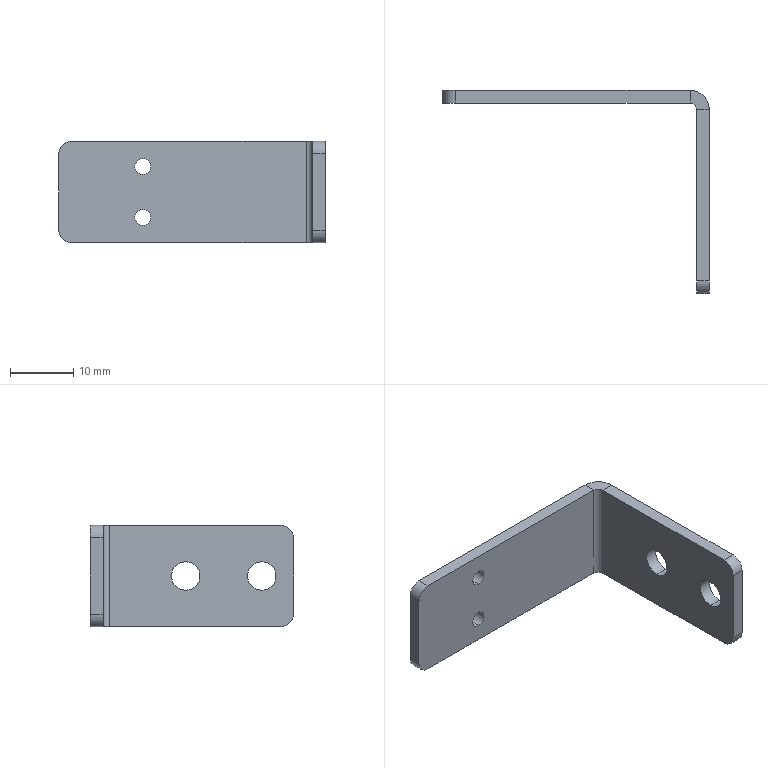Part | NX | features BREP 1 | 1 solid | 26 faces | box 42 x 32 x 16 mm | volume 2186 mm3 | cylinder 14 | plane 12 | commonest cylinder face diameters 2.5 x4 4 x4 4.5 x4 2 x1 6 x1
STEP:
#1=CARTESIAN_POINT('',(-38.,0.,8.));
#2=VERTEX_POINT('',#1);
#3=CARTESIAN_POINT('',(-40.,0.,6.));
#4=VERTEX_POINT('',#3);
#5=CARTESIAN_POINT('',(-38.,0.,6.));
#6=DIRECTION('',(0.,-1.,0.));
#7=DIRECTION('',(1.,0.,0.));
#8=AXIS2_PLACEMENT_3D('',#5,#6,#7);
#9=CIRCLE('',#8,2.);
#10=EDGE_CURVE('',#2,#4,#9,.T.);
#11=ORIENTED_EDGE('',*,*,#10,.F.);
#12=CARTESIAN_POINT('',(-38.,2.,8.));
#13=VERTEX_POINT('',#12);
#14=CARTESIAN_POINT('',(-38.,-1.,8.));
#15=DIRECTION('',(0.,-1.,0.));
#16=VECTOR('',#15,1000.);
#17=LINE('',#14,#16);
#18=EDGE_CURVE('',#13,#2,#17,.T.);
#19=ORIENTED_EDGE('',*,*,#18,.F.);
#20=CARTESIAN_POINT('',(-40.,2.,6.));
#21=VERTEX_POINT('',#20);
#22=CARTESIAN_POINT('',(-38.,2.,6.));
#23=DIRECTION('',(0.,1.,0.));
#24=DIRECTION('',(1.,0.,0.));
#25=AXIS2_PLACEMENT_3D('',#22,#23,#24);
#26=CIRCLE('',#25,2.);
#27=EDGE_CURVE('',#21,#13,#26,.T.);
#28=ORIENTED_EDGE('',*,*,#27,.F.);
#29=CARTESIAN_POINT('',(-40.,0.,6.));
#30=DIRECTION('',(0.,1.,0.));
#31=VECTOR('',#30,1000.);
#32=LINE('',#29,#31);
#33=EDGE_CURVE('',#4,#21,#32,.T.);
#34=ORIENTED_EDGE('',*,*,#33,.F.);
#35=EDGE_LOOP('',(#11,#19,#28,#34));
#36=FACE_BOUND('',#35,.T.);
#37=CARTESIAN_POINT('',(-38.,0.,6.));
#38=DIRECTION('',(0.,1.,0.));
#39=DIRECTION('',(0.,0.,1.));
#40=AXIS2_PLACEMENT_3D('',#37,#38,#39);
#41=CYLINDRICAL_SURFACE('',#40,2.);
#42=ADVANCED_FACE('',(#36),#41,.T.);
#43=CARTESIAN_POINT('',(-40.,0.,-6.));
#44=VERTEX_POINT('',#43);
#45=CARTESIAN_POINT('',(-38.,0.,-8.));
#46=VERTEX_POINT('',#45);
#47=CARTESIAN_POINT('',(-38.,0.,-6.));
#48=DIRECTION('',(0.,-1.,0.));
#49=DIRECTION('',(1.,0.,0.));
#50=AXIS2_PLACEMENT_3D('',#47,#48,#49);
#51=CIRCLE('',#50,2.);
#52=EDGE_CURVE('',#44,#46,#51,.T.);
#53=ORIENTED_EDGE('',*,*,#52,.F.);
#54=CARTESIAN_POINT('',(-40.,2.,-6.));
#55=VERTEX_POINT('',#54);
#56=CARTESIAN_POINT('',(-40.,0.,-6.));
#57=DIRECTION('',(0.,-1.,0.));
#58=VECTOR('',#57,1000.);
#59=LINE('',#56,#58);
#60=EDGE_CURVE('',#55,#44,#59,.T.);
#61=ORIENTED_EDGE('',*,*,#60,.F.);
#62=CARTESIAN_POINT('',(-38.,2.,-8.));
#63=VERTEX_POINT('',#62);
#64=CARTESIAN_POINT('',(-38.,2.,-6.));
#65=DIRECTION('',(0.,1.,0.));
#66=DIRECTION('',(1.,0.,0.));
#67=AXIS2_PLACEMENT_3D('',#64,#65,#66);
#68=CIRCLE('',#67,2.);
#69=EDGE_CURVE('',#63,#55,#68,.T.);
#70=ORIENTED_EDGE('',*,*,#69,.F.);
#71=CARTESIAN_POINT('',(-38.,-1.,-8.));
#72=DIRECTION('',(0.,1.,0.));
#73=VECTOR('',#72,1000.);
#74=LINE('',#71,#73);
#75=EDGE_CURVE('',#46,#63,#74,.T.);
#76=ORIENTED_EDGE('',*,*,#75,.F.);
#77=EDGE_LOOP('',(#53,#61,#70,#76));
#78=FACE_BOUND('',#77,.T.);
#79=CARTESIAN_POINT('',(-38.,-1.,-6.));
#80=DIRECTION('',(0.,1.,0.));
#81=DIRECTION('',(0.,0.,1.));
#82=AXIS2_PLACEMENT_3D('',#79,#80,#81);
#83=CYLINDRICAL_SURFACE('',#82,2.);
#84=ADVANCED_FACE('',(#78),#83,.T.);
#85=CARTESIAN_POINT('',(2.,-28.,8.));
#86=VERTEX_POINT('',#85);
#87=CARTESIAN_POINT('',(2.,-30.,6.));
#88=VERTEX_POINT('',#87);
#89=CARTESIAN_POINT('',(2.,-28.,6.));
#90=DIRECTION('',(1.,0.,0.));
#91=DIRECTION('',(0.,0.,1.));
#92=AXIS2_PLACEMENT_3D('',#89,#90,#91);
#93=CIRCLE('',#92,2.);
#94=EDGE_CURVE('',#86,#88,#93,.T.);
#95=ORIENTED_EDGE('',*,*,#94,.F.);
#96=CARTESIAN_POINT('',(0.,-28.,8.));
#97=VERTEX_POINT('',#96);
#98=CARTESIAN_POINT('',(2.,-28.,8.));
#99=DIRECTION('',(1.,0.,0.));
#100=VECTOR('',#99,1000.);
#101=LINE('',#98,#100);
#102=EDGE_CURVE('',#97,#86,#101,.T.);
#103=ORIENTED_EDGE('',*,*,#102,.F.);
#104=CARTESIAN_POINT('',(0.,-30.,6.));
#105=VERTEX_POINT('',#104);
#106=CARTESIAN_POINT('',(0.,-28.,6.));
#107=DIRECTION('',(-1.,0.,0.));
#108=DIRECTION('',(0.,0.,1.));
#109=AXIS2_PLACEMENT_3D('',#106,#107,#108);
#110=CIRCLE('',#109,2.);
#111=EDGE_CURVE('',#105,#97,#110,.T.);
#112=ORIENTED_EDGE('',*,*,#111,.F.);
#113=CARTESIAN_POINT('',(0.,-30.,6.));
#114=DIRECTION('',(-1.,0.,0.));
#115=VECTOR('',#114,1000.);
#116=LINE('',#113,#115);
#117=EDGE_CURVE('',#88,#105,#116,.T.);
#118=ORIENTED_EDGE('',*,*,#117,.F.);
#119=EDGE_LOOP('',(#95,#103,#112,#118));
#120=FACE_BOUND('',#119,.T.);
#121=CARTESIAN_POINT('',(2.,-28.,6.));
#122=DIRECTION('',(1.,0.,0.));
#123=DIRECTION('',(0.,0.,-1.));
#124=AXIS2_PLACEMENT_3D('',#121,#122,#123);
#125=CYLINDRICAL_SURFACE('',#124,2.);
#126=ADVANCED_FACE('',(#120),#125,.T.);
#127=CARTESIAN_POINT('',(2.,-30.,-6.));
#128=VERTEX_POINT('',#127);
#129=CARTESIAN_POINT('',(2.,-28.,-8.));
#130=VERTEX_POINT('',#129);
#131=CARTESIAN_POINT('',(2.,-28.,-6.));
#132=DIRECTION('',(1.,0.,0.));
#133=DIRECTION('',(0.,0.,1.));
#134=AXIS2_PLACEMENT_3D('',#131,#132,#133);
#135=CIRCLE('',#134,2.);
#136=EDGE_CURVE('',#128,#130,#135,.T.);
#137=ORIENTED_EDGE('',*,*,#136,.F.);
#138=CARTESIAN_POINT('',(0.,-30.,-6.));
#139=VERTEX_POINT('',#138);
#140=CARTESIAN_POINT('',(2.,-30.,-6.));
#141=DIRECTION('',(1.,0.,0.));
#142=VECTOR('',#141,1000.);
#143=LINE('',#140,#142);
#144=EDGE_CURVE('',#139,#128,#143,.T.);
#145=ORIENTED_EDGE('',*,*,#144,.F.);
#146=CARTESIAN_POINT('',(0.,-28.,-8.));
#147=VERTEX_POINT('',#146);
#148=CARTESIAN_POINT('',(0.,-28.,-6.));
#149=DIRECTION('',(-1.,0.,0.));
#150=DIRECTION('',(0.,0.,1.));
#151=AXIS2_PLACEMENT_3D('',#148,#149,#150);
#152=CIRCLE('',#151,2.);
#153=EDGE_CURVE('',#147,#139,#152,.T.);
#154=ORIENTED_EDGE('',*,*,#153,.F.);
#155=CARTESIAN_POINT('',(-1.,-28.,-8.));
#156=DIRECTION('',(-1.,0.,0.));
#157=VECTOR('',#156,1000.);
#158=LINE('',#155,#157);
#159=EDGE_CURVE('',#130,#147,#158,.T.);
#160=ORIENTED_EDGE('',*,*,#159,.F.);
#161=EDGE_LOOP('',(#137,#145,#154,#160));
#162=FACE_BOUND('',#161,.T.);
#163=CARTESIAN_POINT('',(-1.,-28.,-6.));
#164=DIRECTION('',(-1.,0.,0.));
#165=DIRECTION('',(0.,0.,1.));
#166=AXIS2_PLACEMENT_3D('',#163,#164,#165);
#167=CYLINDRICAL_SURFACE('',#166,2.);
#168=ADVANCED_FACE('',(#162),#167,.T.);
#169=CARTESIAN_POINT('',(0.,-13.,-2.25));
#170=VERTEX_POINT('',#169);
#171=CARTESIAN_POINT('',(2.,-13.,-2.25));
#172=VERTEX_POINT('',#171);
#173=CARTESIAN_POINT('',(0.,-13.,-2.25));
#174=DIRECTION('',(-1.,0.,0.));
#175=VECTOR('',#174,1000.);
#176=LINE('',#173,#175);
#177=EDGE_CURVE('',#170,#172,#176,.F.);
#178=ORIENTED_EDGE('',*,*,#177,.T.);
#179=CARTESIAN_POINT('',(2.,-13.,2.25));
#180=VERTEX_POINT('',#179);
#181=CARTESIAN_POINT('',(2.,-13.,0.));
#182=DIRECTION('',(-1.,0.,0.));
#183=DIRECTION('',(0.,0.,1.));
#184=AXIS2_PLACEMENT_3D('',#181,#182,#183);
#185=CIRCLE('',#184,2.25);
#186=EDGE_CURVE('',#180,#172,#185,.T.);
#187=ORIENTED_EDGE('',*,*,#186,.F.);
#188=CARTESIAN_POINT('',(0.,-13.,2.25));
#189=VERTEX_POINT('',#188);
#190=CARTESIAN_POINT('',(0.,-13.,2.25));
#191=DIRECTION('',(-1.,0.,0.));
#192=VECTOR('',#191,1000.);
#193=LINE('',#190,#192);
#194=EDGE_CURVE('',#189,#180,#193,.F.);
#195=ORIENTED_EDGE('',*,*,#194,.F.);
#196=CARTESIAN_POINT('',(0.,-13.,0.));
#197=DIRECTION('',(-1.,0.,0.));
#198=DIRECTION('',(0.,0.,1.));
#199=AXIS2_PLACEMENT_3D('',#196,#197,#198);
#200=CIRCLE('',#199,2.25);
#201=EDGE_CURVE('',#189,#170,#200,.T.);
#202=ORIENTED_EDGE('',*,*,#201,.T.);
#203=EDGE_LOOP('',(#178,#187,#195,#202));
#204=FACE_BOUND('',#203,.T.);
#205=CARTESIAN_POINT('',(0.,-13.,0.));
#206=DIRECTION('',(-1.,0.,0.));
#207=DIRECTION('',(0.,0.,1.));
#208=AXIS2_PLACEMENT_3D('',#205,#206,#207);
#209=CYLINDRICAL_SURFACE('',#208,2.25);
#210=ADVANCED_FACE('',(#204),#209,.F.);
#211=CARTESIAN_POINT('',(0.,-25.,-2.25));
#212=VERTEX_POINT('',#211);
#213=CARTESIAN_POINT('',(2.,-25.,-2.25));
#214=VERTEX_POINT('',#213);
#215=CARTESIAN_POINT('',(0.,-25.,-2.25));
#216=DIRECTION('',(-1.,0.,0.));
#217=VECTOR('',#216,1000.);
#218=LINE('',#215,#217);
#219=EDGE_CURVE('',#212,#214,#218,.F.);
#220=ORIENTED_EDGE('',*,*,#219,.T.);
#221=CARTESIAN_POINT('',(2.,-25.,2.25));
#222=VERTEX_POINT('',#221);
#223=CARTESIAN_POINT('',(2.,-25.,0.));
#224=DIRECTION('',(-1.,0.,0.));
#225=DIRECTION('',(0.,0.,1.));
#226=AXIS2_PLACEMENT_3D('',#223,#224,#225);
#227=CIRCLE('',#226,2.25);
#228=EDGE_CURVE('',#222,#214,#227,.T.);
#229=ORIENTED_EDGE('',*,*,#228,.F.);
#230=CARTESIAN_POINT('',(0.,-25.,2.25));
#231=VERTEX_POINT('',#230);
#232=CARTESIAN_POINT('',(0.,-25.,2.25));
#233=DIRECTION('',(-1.,0.,0.));
#234=VECTOR('',#233,1000.);
#235=LINE('',#232,#234);
#236=EDGE_CURVE('',#231,#222,#235,.F.);
#237=ORIENTED_EDGE('',*,*,#236,.F.);
#238=CARTESIAN_POINT('',(0.,-25.,0.));
#239=DIRECTION('',(-1.,0.,0.));
#240=DIRECTION('',(0.,0.,1.));
#241=AXIS2_PLACEMENT_3D('',#238,#239,#240);
#242=CIRCLE('',#241,2.25);
#243=EDGE_CURVE('',#231,#212,#242,.T.);
#244=ORIENTED_EDGE('',*,*,#243,.T.);
#245=EDGE_LOOP('',(#220,#229,#237,#244));
#246=FACE_BOUND('',#245,.T.);
#247=CARTESIAN_POINT('',(0.,-25.,0.));
#248=DIRECTION('',(-1.,0.,0.));
#249=DIRECTION('',(0.,0.,1.));
#250=AXIS2_PLACEMENT_3D('',#247,#248,#249);
#251=CYLINDRICAL_SURFACE('',#250,2.25);
#252=ADVANCED_FACE('',(#246),#251,.F.);
#253=CARTESIAN_POINT('',(-26.75,2.,2.75));
#254=VERTEX_POINT('',#253);
#255=CARTESIAN_POINT('',(-26.75,0.,2.75));
#256=VERTEX_POINT('',#255);
#257=CARTESIAN_POINT('',(-26.75,2.,2.75));
#258=DIRECTION('',(0.,1.,0.));
#259=VECTOR('',#258,1000.);
#260=LINE('',#257,#259);
#261=EDGE_CURVE('',#254,#256,#260,.F.);
#262=ORIENTED_EDGE('',*,*,#261,.T.);
#263=CARTESIAN_POINT('',(-26.75,0.,5.25));
#264=VERTEX_POINT('',#263);
#265=CARTESIAN_POINT('',(-26.75,0.,4.));
#266=DIRECTION('',(0.,-1.,0.));
#267=DIRECTION('',(1.,0.,0.));
#268=AXIS2_PLACEMENT_3D('',#265,#266,#267);
#269=CIRCLE('',#268,1.25);
#270=EDGE_CURVE('',#256,#264,#269,.T.);
#271=ORIENTED_EDGE('',*,*,#270,.T.);
#272=CARTESIAN_POINT('',(-26.75,2.,5.25));
#273=VERTEX_POINT('',#272);
#274=CARTESIAN_POINT('',(-26.75,2.,5.25));
#275=DIRECTION('',(0.,1.,0.));
#276=VECTOR('',#275,1000.);
#277=LINE('',#274,#276);
#278=EDGE_CURVE('',#273,#264,#277,.F.);
#279=ORIENTED_EDGE('',*,*,#278,.F.);
#280=CARTESIAN_POINT('',(-26.75,2.,4.));
#281=DIRECTION('',(0.,1.,0.));
#282=DIRECTION('',(0.,0.,1.));
#283=AXIS2_PLACEMENT_3D('',#280,#281,#282);
#284=CIRCLE('',#283,1.25);
#285=EDGE_CURVE('',#273,#254,#284,.T.);
#286=ORIENTED_EDGE('',*,*,#285,.T.);
#287=EDGE_LOOP('',(#262,#271,#279,#286));
#288=FACE_BOUND('',#287,.T.);
#289=CARTESIAN_POINT('',(-26.75,2.,4.));
#290=DIRECTION('',(0.,1.,0.));
#291=DIRECTION('',(0.,0.,1.));
#292=AXIS2_PLACEMENT_3D('',#289,#290,#291);
#293=CYLINDRICAL_SURFACE('',#292,1.25);
#294=ADVANCED_FACE('',(#288),#293,.F.);
#295=CARTESIAN_POINT('',(-26.75,2.,-5.25));
#296=VERTEX_POINT('',#295);
#297=CARTESIAN_POINT('',(-26.75,0.,-5.25));
#298=VERTEX_POINT('',#297);
#299=CARTESIAN_POINT('',(-26.75,2.,-5.25));
#300=DIRECTION('',(0.,1.,0.));
#301=VECTOR('',#300,1000.);
#302=LINE('',#299,#301);
#303=EDGE_CURVE('',#296,#298,#302,.F.);
#304=ORIENTED_EDGE('',*,*,#303,.T.);
#305=CARTESIAN_POINT('',(-26.75,0.,-2.75));
#306=VERTEX_POINT('',#305);
#307=CARTESIAN_POINT('',(-26.75,0.,-4.));
#308=DIRECTION('',(0.,-1.,0.));
#309=DIRECTION('',(1.,0.,0.));
#310=AXIS2_PLACEMENT_3D('',#307,#308,#309);
#311=CIRCLE('',#310,1.25);
#312=EDGE_CURVE('',#298,#306,#311,.T.);
#313=ORIENTED_EDGE('',*,*,#312,.T.);
#314=CARTESIAN_POINT('',(-26.75,2.,-2.75));
#315=VERTEX_POINT('',#314);
#316=CARTESIAN_POINT('',(-26.75,2.,-2.75));
#317=DIRECTION('',(0.,1.,0.));
#318=VECTOR('',#317,1000.);
#319=LINE('',#316,#318);
#320=EDGE_CURVE('',#315,#306,#319,.F.);
#321=ORIENTED_EDGE('',*,*,#320,.F.);
#322=CARTESIAN_POINT('',(-26.75,2.,-4.));
#323=DIRECTION('',(0.,1.,0.));
#324=DIRECTION('',(0.,0.,1.));
#325=AXIS2_PLACEMENT_3D('',#322,#323,#324);
#326=CIRCLE('',#325,1.25);
#327=EDGE_CURVE('',#315,#296,#326,.T.);
#328=ORIENTED_EDGE('',*,*,#327,.T.);
#329=EDGE_LOOP('',(#304,#313,#321,#328));
#330=FACE_BOUND('',#329,.T.);
#331=CARTESIAN_POINT('',(-26.75,2.,-4.));
#332=DIRECTION('',(0.,1.,0.));
#333=DIRECTION('',(0.,0.,1.));
#334=AXIS2_PLACEMENT_3D('',#331,#332,#333);
#335=CYLINDRICAL_SURFACE('',#334,1.25);
#336=ADVANCED_FACE('',(#330),#335,.F.);
#337=CARTESIAN_POINT('',(-1.,0.,-8.));
#338=VERTEX_POINT('',#337);
#339=CARTESIAN_POINT('',(0.,0.,-8.));
#340=DIRECTION('',(-1.,0.,0.));
#341=VECTOR('',#340,1000.);
#342=LINE('',#339,#341);
#343=EDGE_CURVE('',#338,#46,#342,.T.);
#344=ORIENTED_EDGE('',*,*,#343,.T.);
#345=ORIENTED_EDGE('',*,*,#75,.T.);
#346=CARTESIAN_POINT('',(-1.,2.,-8.));
#347=VERTEX_POINT('',#346);
#348=CARTESIAN_POINT('',(0.,2.,-8.));
#349=DIRECTION('',(-1.,0.,0.));
#350=VECTOR('',#349,1000.);
#351=LINE('',#348,#350);
#352=EDGE_CURVE('',#347,#63,#351,.T.);
#353=ORIENTED_EDGE('',*,*,#352,.F.);
#354=CARTESIAN_POINT('',(-1.,2.,-8.));
#355=DIRECTION('',(0.,-1.,0.));
#356=VECTOR('',#355,1000.);
#357=LINE('',#354,#356);
#358=EDGE_CURVE('',#347,#338,#357,.T.);
#359=ORIENTED_EDGE('',*,*,#358,.T.);
#360=EDGE_LOOP('',(#344,#345,#353,#359));
#361=FACE_BOUND('',#360,.T.);
#362=CARTESIAN_POINT('',(-1.,-1.,-8.));
#363=DIRECTION('',(0.,0.,-1.));
#364=DIRECTION('',(-1.,0.,0.));
#365=AXIS2_PLACEMENT_3D('',#362,#363,#364);
#366=PLANE('',#365);
#367=ADVANCED_FACE('',(#361),#366,.T.);
#368=CARTESIAN_POINT('',(0.,-1.,8.));
#369=VERTEX_POINT('',#368);
#370=CARTESIAN_POINT('',(0.,0.,8.));
#371=DIRECTION('',(0.,1.,0.));
#372=VECTOR('',#371,1000.);
#373=LINE('',#370,#372);
#374=EDGE_CURVE('',#97,#369,#373,.T.);
#375=ORIENTED_EDGE('',*,*,#374,.F.);
#376=ORIENTED_EDGE('',*,*,#102,.T.);
#377=CARTESIAN_POINT('',(2.,-1.,8.));
#378=VERTEX_POINT('',#377);
#379=CARTESIAN_POINT('',(2.,0.,8.));
#380=DIRECTION('',(0.,1.,0.));
#381=VECTOR('',#380,1000.);
#382=LINE('',#379,#381);
#383=EDGE_CURVE('',#86,#378,#382,.T.);
#384=ORIENTED_EDGE('',*,*,#383,.T.);
#385=CARTESIAN_POINT('',(2.,-1.,8.));
#386=DIRECTION('',(-1.,0.,0.));
#387=VECTOR('',#386,1000.);
#388=LINE('',#385,#387);
#389=EDGE_CURVE('',#378,#369,#388,.T.);
#390=ORIENTED_EDGE('',*,*,#389,.T.);
#391=EDGE_LOOP('',(#375,#376,#384,#390));
#392=FACE_BOUND('',#391,.T.);
#393=CARTESIAN_POINT('',(-1.,-1.,8.));
#394=DIRECTION('',(0.,0.,-1.));
#395=DIRECTION('',(-1.,0.,0.));
#396=AXIS2_PLACEMENT_3D('',#393,#394,#395);
#397=PLANE('',#396);
#398=ADVANCED_FACE('',(#392),#397,.F.);
#399=CARTESIAN_POINT('',(2.,-1.,-8.));
#400=VERTEX_POINT('',#399);
#401=CARTESIAN_POINT('',(-1.,-1.,-8.));
#402=DIRECTION('',(0.,0.,1.));
#403=DIRECTION('',(1.,0.,0.));
#404=AXIS2_PLACEMENT_3D('',#401,#402,#403);
#405=CIRCLE('',#404,3.);
#406=EDGE_CURVE('',#400,#347,#405,.T.);
#407=ORIENTED_EDGE('',*,*,#406,.T.);
#408=CARTESIAN_POINT('',(-1.,2.,8.));
#409=VERTEX_POINT('',#408);
#410=CARTESIAN_POINT('',(-1.,2.,8.));
#411=DIRECTION('',(0.,0.,-1.));
#412=VECTOR('',#411,1000.);
#413=LINE('',#410,#412);
#414=EDGE_CURVE('',#409,#347,#413,.T.);
#415=ORIENTED_EDGE('',*,*,#414,.F.);
#416=CARTESIAN_POINT('',(-1.,-1.,8.));
#417=DIRECTION('',(0.,0.,1.));
#418=DIRECTION('',(1.,0.,0.));
#419=AXIS2_PLACEMENT_3D('',#416,#417,#418);
#420=CIRCLE('',#419,3.);
#421=EDGE_CURVE('',#378,#409,#420,.T.);
#422=ORIENTED_EDGE('',*,*,#421,.F.);
#423=CARTESIAN_POINT('',(2.,-1.,8.));
#424=DIRECTION('',(0.,0.,-1.));
#425=VECTOR('',#424,1000.);
#426=LINE('',#423,#425);
#427=EDGE_CURVE('',#378,#400,#426,.T.);
#428=ORIENTED_EDGE('',*,*,#427,.T.);
#429=EDGE_LOOP('',(#407,#415,#422,#428));
#430=FACE_BOUND('',#429,.T.);
#431=CARTESIAN_POINT('',(-1.,-1.,8.));
#432=DIRECTION('',(0.,0.,-1.));
#433=DIRECTION('',(-1.,0.,0.));
#434=AXIS2_PLACEMENT_3D('',#431,#432,#433);
#435=CYLINDRICAL_SURFACE('',#434,3.);
#436=ADVANCED_FACE('',(#430),#435,.T.);
#437=CARTESIAN_POINT('',(2.,-30.,8.));
#438=DIRECTION('',(0.,0.,-1.));
#439=VECTOR('',#438,1000.);
#440=LINE('',#437,#439);
#441=EDGE_CURVE('',#88,#128,#440,.T.);
#442=ORIENTED_EDGE('',*,*,#441,.T.);
#443=ORIENTED_EDGE('',*,*,#136,.T.);
#444=CARTESIAN_POINT('',(2.,0.,-8.));
#445=DIRECTION('',(0.,1.,0.));
#446=VECTOR('',#445,1000.);
#447=LINE('',#444,#446);
#448=EDGE_CURVE('',#130,#400,#447,.T.);
#449=ORIENTED_EDGE('',*,*,#448,.T.);
#450=ORIENTED_EDGE('',*,*,#427,.F.);
#451=ORIENTED_EDGE('',*,*,#383,.F.);
#452=ORIENTED_EDGE('',*,*,#94,.T.);
#453=EDGE_LOOP('',(#442,#443,#449,#450,#451,#452));
#454=FACE_BOUND('',#453,.T.);
#455=ORIENTED_EDGE('',*,*,#228,.T.);
#456=CARTESIAN_POINT('',(2.,-25.,0.));
#457=DIRECTION('',(-1.,0.,0.));
#458=DIRECTION('',(0.,0.,1.));
#459=AXIS2_PLACEMENT_3D('',#456,#457,#458);
#460=CIRCLE('',#459,2.25);
#461=EDGE_CURVE('',#214,#222,#460,.T.);
#462=ORIENTED_EDGE('',*,*,#461,.T.);
#463=EDGE_LOOP('',(#455,#462));
#464=FACE_BOUND('',#463,.T.);
#465=ORIENTED_EDGE('',*,*,#186,.T.);
#466=CARTESIAN_POINT('',(2.,-13.,0.));
#467=DIRECTION('',(-1.,0.,0.));
#468=DIRECTION('',(0.,0.,1.));
#469=AXIS2_PLACEMENT_3D('',#466,#467,#468);
#470=CIRCLE('',#469,2.25);
#471=EDGE_CURVE('',#172,#180,#470,.T.);
#472=ORIENTED_EDGE('',*,*,#471,.T.);
#473=EDGE_LOOP('',(#465,#472));
#474=FACE_BOUND('',#473,.T.);
#475=CARTESIAN_POINT('',(2.,0.,8.));
#476=DIRECTION('',(-1.,0.,0.));
#477=DIRECTION('',(0.,0.,1.));
#478=AXIS2_PLACEMENT_3D('',#475,#476,#477);
#479=PLANE('',#478);
#480=ADVANCED_FACE('',(#454,#464,#474),#479,.F.);
#481=CARTESIAN_POINT('',(0.,-30.,8.));
#482=DIRECTION('',(0.,0.,-1.));
#483=VECTOR('',#482,1000.);
#484=LINE('',#481,#483);
#485=EDGE_CURVE('',#105,#139,#484,.T.);
#486=ORIENTED_EDGE('',*,*,#485,.T.);
#487=ORIENTED_EDGE('',*,*,#144,.T.);
#488=ORIENTED_EDGE('',*,*,#441,.F.);
#489=ORIENTED_EDGE('',*,*,#117,.T.);
#490=EDGE_LOOP('',(#486,#487,#488,#489));
#491=FACE_BOUND('',#490,.T.);
#492=CARTESIAN_POINT('',(2.,-30.,8.));
#493=DIRECTION('',(0.,-1.,0.));
#494=DIRECTION('',(0.,0.,-1.));
#495=AXIS2_PLACEMENT_3D('',#492,#493,#494);
#496=PLANE('',#495);
#497=ADVANCED_FACE('',(#491),#496,.T.);
#498=CARTESIAN_POINT('',(0.,-1.,-8.));
#499=VERTEX_POINT('',#498);
#500=CARTESIAN_POINT('',(0.,0.,-8.));
#501=DIRECTION('',(0.,1.,0.));
#502=VECTOR('',#501,1000.);
#503=LINE('',#500,#502);
#504=EDGE_CURVE('',#147,#499,#503,.T.);
#505=ORIENTED_EDGE('',*,*,#504,.F.);
#506=ORIENTED_EDGE('',*,*,#153,.T.);
#507=ORIENTED_EDGE('',*,*,#485,.F.);
#508=ORIENTED_EDGE('',*,*,#111,.T.);
#509=ORIENTED_EDGE('',*,*,#374,.T.);
#510=CARTESIAN_POINT('',(0.,-1.,8.));
#511=DIRECTION('',(0.,0.,-1.));
#512=VECTOR('',#511,1000.);
#513=LINE('',#510,#512);
#514=EDGE_CURVE('',#369,#499,#513,.T.);
#515=ORIENTED_EDGE('',*,*,#514,.T.);
#516=EDGE_LOOP('',(#505,#506,#507,#508,#509,#515));
#517=FACE_BOUND('',#516,.T.);
#518=ORIENTED_EDGE('',*,*,#243,.F.);
#519=CARTESIAN_POINT('',(0.,-25.,0.));
#520=DIRECTION('',(-1.,0.,0.));
#521=DIRECTION('',(0.,0.,1.));
#522=AXIS2_PLACEMENT_3D('',#519,#520,#521);
#523=CIRCLE('',#522,2.25);
#524=EDGE_CURVE('',#212,#231,#523,.T.);
#525=ORIENTED_EDGE('',*,*,#524,.F.);
#526=EDGE_LOOP('',(#518,#525));
#527=FACE_BOUND('',#526,.T.);
#528=ORIENTED_EDGE('',*,*,#201,.F.);
#529=CARTESIAN_POINT('',(0.,-13.,0.));
#530=DIRECTION('',(-1.,0.,0.));
#531=DIRECTION('',(0.,0.,1.));
#532=AXIS2_PLACEMENT_3D('',#529,#530,#531);
#533=CIRCLE('',#532,2.25);
#534=EDGE_CURVE('',#170,#189,#533,.T.);
#535=ORIENTED_EDGE('',*,*,#534,.F.);
#536=EDGE_LOOP('',(#528,#535));
#537=FACE_BOUND('',#536,.T.);
#538=CARTESIAN_POINT('',(0.,0.,8.));
#539=DIRECTION('',(-1.,0.,0.));
#540=DIRECTION('',(0.,0.,1.));
#541=AXIS2_PLACEMENT_3D('',#538,#539,#540);
#542=PLANE('',#541);
#543=ADVANCED_FACE('',(#517,#527,#537),#542,.T.);
#544=CARTESIAN_POINT('',(-1.,-1.,-8.));
#545=DIRECTION('',(0.,0.,1.));
#546=DIRECTION('',(-1.,0.,0.));
#547=AXIS2_PLACEMENT_3D('',#544,#545,#546);
#548=CIRCLE('',#547,1.);
#549=EDGE_CURVE('',#499,#338,#548,.T.);
#550=ORIENTED_EDGE('',*,*,#549,.F.);
#551=ORIENTED_EDGE('',*,*,#514,.F.);
#552=CARTESIAN_POINT('',(-1.,0.,8.));
#553=VERTEX_POINT('',#552);
#554=CARTESIAN_POINT('',(-1.,-1.,8.));
#555=DIRECTION('',(0.,0.,1.));
#556=DIRECTION('',(-1.,0.,0.));
#557=AXIS2_PLACEMENT_3D('',#554,#555,#556);
#558=CIRCLE('',#557,1.);
#559=EDGE_CURVE('',#369,#553,#558,.T.);
#560=ORIENTED_EDGE('',*,*,#559,.T.);
#561=CARTESIAN_POINT('',(-1.,0.,8.));
#562=DIRECTION('',(0.,0.,-1.));
#563=VECTOR('',#562,1000.);
#564=LINE('',#561,#563);
#565=EDGE_CURVE('',#553,#338,#564,.T.);
#566=ORIENTED_EDGE('',*,*,#565,.T.);
#567=EDGE_LOOP('',(#550,#551,#560,#566));
#568=FACE_BOUND('',#567,.T.);
#569=CARTESIAN_POINT('',(-1.,-1.,8.));
#570=DIRECTION('',(0.,0.,-1.));
#571=DIRECTION('',(-1.,0.,0.));
#572=AXIS2_PLACEMENT_3D('',#569,#570,#571);
#573=CYLINDRICAL_SURFACE('',#572,1.);
#574=ADVANCED_FACE('',(#568),#573,.F.);
#575=CARTESIAN_POINT('',(-40.,0.,8.));
#576=DIRECTION('',(0.,0.,-1.));
#577=VECTOR('',#576,1000.);
#578=LINE('',#575,#577);
#579=EDGE_CURVE('',#4,#44,#578,.T.);
#580=ORIENTED_EDGE('',*,*,#579,.T.);
#581=ORIENTED_EDGE('',*,*,#52,.T.);
#582=ORIENTED_EDGE('',*,*,#343,.F.);
#583=ORIENTED_EDGE('',*,*,#565,.F.);
#584=CARTESIAN_POINT('',(0.,0.,8.));
#585=DIRECTION('',(-1.,0.,0.));
#586=VECTOR('',#585,1000.);
#587=LINE('',#584,#586);
#588=EDGE_CURVE('',#553,#2,#587,.T.);
#589=ORIENTED_EDGE('',*,*,#588,.T.);
#590=ORIENTED_EDGE('',*,*,#10,.T.);
#591=EDGE_LOOP('',(#580,#581,#582,#583,#589,#590));
#592=FACE_BOUND('',#591,.T.);
#593=CARTESIAN_POINT('',(-26.75,0.,-4.));
#594=DIRECTION('',(0.,-1.,0.));
#595=DIRECTION('',(1.,0.,0.));
#596=AXIS2_PLACEMENT_3D('',#593,#594,#595);
#597=CIRCLE('',#596,1.25);
#598=EDGE_CURVE('',#306,#298,#597,.T.);
#599=ORIENTED_EDGE('',*,*,#598,.F.);
#600=ORIENTED_EDGE('',*,*,#312,.F.);
#601=EDGE_LOOP('',(#599,#600));
#602=FACE_BOUND('',#601,.T.);
#603=CARTESIAN_POINT('',(-26.75,0.,4.));
#604=DIRECTION('',(0.,-1.,0.));
#605=DIRECTION('',(1.,0.,0.));
#606=AXIS2_PLACEMENT_3D('',#603,#604,#605);
#607=CIRCLE('',#606,1.25);
#608=EDGE_CURVE('',#264,#256,#607,.T.);
#609=ORIENTED_EDGE('',*,*,#608,.F.);
#610=ORIENTED_EDGE('',*,*,#270,.F.);
#611=EDGE_LOOP('',(#609,#610));
#612=FACE_BOUND('',#611,.T.);
#613=CARTESIAN_POINT('',(0.,0.,8.));
#614=DIRECTION('',(0.,-1.,0.));
#615=DIRECTION('',(1.,0.,0.));
#616=AXIS2_PLACEMENT_3D('',#613,#614,#615);
#617=PLANE('',#616);
#618=ADVANCED_FACE('',(#592,#602,#612),#617,.T.);
#619=CARTESIAN_POINT('',(-40.,2.,8.));
#620=DIRECTION('',(0.,0.,-1.));
#621=VECTOR('',#620,1000.);
#622=LINE('',#619,#621);
#623=EDGE_CURVE('',#21,#55,#622,.T.);
#624=ORIENTED_EDGE('',*,*,#623,.T.);
#625=ORIENTED_EDGE('',*,*,#60,.T.);
#626=ORIENTED_EDGE('',*,*,#579,.F.);
#627=ORIENTED_EDGE('',*,*,#33,.T.);
#628=EDGE_LOOP('',(#624,#625,#626,#627));
#629=FACE_BOUND('',#628,.T.);
#630=CARTESIAN_POINT('',(-40.,0.,8.));
#631=DIRECTION('',(-1.,0.,0.));
#632=DIRECTION('',(0.,0.,1.));
#633=AXIS2_PLACEMENT_3D('',#630,#631,#632);
#634=PLANE('',#633);
#635=ADVANCED_FACE('',(#629),#634,.T.);
#636=ORIENTED_EDGE('',*,*,#352,.T.);
#637=ORIENTED_EDGE('',*,*,#69,.T.);
#638=ORIENTED_EDGE('',*,*,#623,.F.);
#639=ORIENTED_EDGE('',*,*,#27,.T.);
#640=CARTESIAN_POINT('',(0.,2.,8.));
#641=DIRECTION('',(-1.,0.,0.));
#642=VECTOR('',#641,1000.);
#643=LINE('',#640,#642);
#644=EDGE_CURVE('',#409,#13,#643,.T.);
#645=ORIENTED_EDGE('',*,*,#644,.F.);
#646=ORIENTED_EDGE('',*,*,#414,.T.);
#647=EDGE_LOOP('',(#636,#637,#638,#639,#645,#646));
#648=FACE_BOUND('',#647,.T.);
#649=ORIENTED_EDGE('',*,*,#327,.F.);
#650=CARTESIAN_POINT('',(-26.75,2.,-4.));
#651=DIRECTION('',(0.,1.,0.));
#652=DIRECTION('',(0.,0.,1.));
#653=AXIS2_PLACEMENT_3D('',#650,#651,#652);
#654=CIRCLE('',#653,1.25);
#655=EDGE_CURVE('',#296,#315,#654,.T.);
#656=ORIENTED_EDGE('',*,*,#655,.F.);
#657=EDGE_LOOP('',(#649,#656));
#658=FACE_BOUND('',#657,.T.);
#659=ORIENTED_EDGE('',*,*,#285,.F.);
#660=CARTESIAN_POINT('',(-26.75,2.,4.));
#661=DIRECTION('',(0.,1.,0.));
#662=DIRECTION('',(0.,0.,1.));
#663=AXIS2_PLACEMENT_3D('',#660,#661,#662);
#664=CIRCLE('',#663,1.25);
#665=EDGE_CURVE('',#254,#273,#664,.T.);
#666=ORIENTED_EDGE('',*,*,#665,.F.);
#667=EDGE_LOOP('',(#659,#666));
#668=FACE_BOUND('',#667,.T.);
#669=CARTESIAN_POINT('',(0.,2.,8.));
#670=DIRECTION('',(0.,-1.,0.));
#671=DIRECTION('',(1.,0.,0.));
#672=AXIS2_PLACEMENT_3D('',#669,#670,#671);
#673=PLANE('',#672);
#674=ADVANCED_FACE('',(#648,#658,#668),#673,.F.);
#675=ORIENTED_EDGE('',*,*,#448,.F.);
#676=ORIENTED_EDGE('',*,*,#159,.T.);
#677=ORIENTED_EDGE('',*,*,#504,.T.);
#678=CARTESIAN_POINT('',(0.,-1.,-8.));
#679=DIRECTION('',(1.,0.,0.));
#680=VECTOR('',#679,1000.);
#681=LINE('',#678,#680);
#682=EDGE_CURVE('',#499,#400,#681,.T.);
#683=ORIENTED_EDGE('',*,*,#682,.T.);
#684=EDGE_LOOP('',(#675,#676,#677,#683));
#685=FACE_BOUND('',#684,.T.);
#686=CARTESIAN_POINT('',(-1.,2.,-8.));
#687=DIRECTION('',(0.,0.,-1.));
#688=DIRECTION('',(-1.,0.,0.));
#689=AXIS2_PLACEMENT_3D('',#686,#687,#688);
#690=PLANE('',#689);
#691=ADVANCED_FACE('',(#685),#690,.T.);
#692=ORIENTED_EDGE('',*,*,#682,.F.);
#693=ORIENTED_EDGE('',*,*,#549,.T.);
#694=ORIENTED_EDGE('',*,*,#358,.F.);
#695=ORIENTED_EDGE('',*,*,#406,.F.);
#696=EDGE_LOOP('',(#692,#693,#694,#695));
#697=FACE_BOUND('',#696,.T.);
#698=CARTESIAN_POINT('',(0.,-1.,-8.));
#699=DIRECTION('',(0.,0.,-1.));
#700=DIRECTION('',(-1.,0.,0.));
#701=AXIS2_PLACEMENT_3D('',#698,#699,#700);
#702=PLANE('',#701);
#703=ADVANCED_FACE('',(#697),#702,.T.);
#704=ORIENTED_EDGE('',*,*,#644,.T.);
#705=ORIENTED_EDGE('',*,*,#18,.T.);
#706=ORIENTED_EDGE('',*,*,#588,.F.);
#707=CARTESIAN_POINT('',(-1.,0.,8.));
#708=DIRECTION('',(0.,1.,0.));
#709=VECTOR('',#708,1000.);
#710=LINE('',#707,#709);
#711=EDGE_CURVE('',#553,#409,#710,.T.);
#712=ORIENTED_EDGE('',*,*,#711,.T.);
#713=EDGE_LOOP('',(#704,#705,#706,#712));
#714=FACE_BOUND('',#713,.T.);
#715=CARTESIAN_POINT('',(2.,-1.,8.));
#716=DIRECTION('',(0.,0.,1.));
#717=DIRECTION('',(1.,0.,0.));
#718=AXIS2_PLACEMENT_3D('',#715,#716,#717);
#719=PLANE('',#718);
#720=ADVANCED_FACE('',(#714),#719,.T.);
#721=ORIENTED_EDGE('',*,*,#711,.F.);
#722=ORIENTED_EDGE('',*,*,#559,.F.);
#723=ORIENTED_EDGE('',*,*,#389,.F.);
#724=ORIENTED_EDGE('',*,*,#421,.T.);
#725=EDGE_LOOP('',(#721,#722,#723,#724));
#726=FACE_BOUND('',#725,.T.);
#727=CARTESIAN_POINT('',(-1.,0.,8.));
#728=DIRECTION('',(0.,0.,1.));
#729=DIRECTION('',(1.,0.,0.));
#730=AXIS2_PLACEMENT_3D('',#727,#728,#729);
#731=PLANE('',#730);
#732=ADVANCED_FACE('',(#726),#731,.T.);
#733=ORIENTED_EDGE('',*,*,#598,.T.);
#734=ORIENTED_EDGE('',*,*,#303,.F.);
#735=ORIENTED_EDGE('',*,*,#655,.T.);
#736=ORIENTED_EDGE('',*,*,#320,.T.);
#737=EDGE_LOOP('',(#733,#734,#735,#736));
#738=FACE_BOUND('',#737,.T.);
#739=CARTESIAN_POINT('',(-26.75,2.,-4.));
#740=DIRECTION('',(0.,1.,0.));
#741=DIRECTION('',(0.,0.,1.));
#742=AXIS2_PLACEMENT_3D('',#739,#740,#741);
#743=CYLINDRICAL_SURFACE('',#742,1.25);
#744=ADVANCED_FACE('',(#738),#743,.F.);
#745=ORIENTED_EDGE('',*,*,#608,.T.);
#746=ORIENTED_EDGE('',*,*,#261,.F.);
#747=ORIENTED_EDGE('',*,*,#665,.T.);
#748=ORIENTED_EDGE('',*,*,#278,.T.);
#749=EDGE_LOOP('',(#745,#746,#747,#748));
#750=FACE_BOUND('',#749,.T.);
#751=CARTESIAN_POINT('',(-26.75,2.,4.));
#752=DIRECTION('',(0.,1.,0.));
#753=DIRECTION('',(0.,0.,1.));
#754=AXIS2_PLACEMENT_3D('',#751,#752,#753);
#755=CYLINDRICAL_SURFACE('',#754,1.25);
#756=ADVANCED_FACE('',(#750),#755,.F.);
#757=ORIENTED_EDGE('',*,*,#461,.F.);
#758=ORIENTED_EDGE('',*,*,#219,.F.);
#759=ORIENTED_EDGE('',*,*,#524,.T.);
#760=ORIENTED_EDGE('',*,*,#236,.T.);
#761=EDGE_LOOP('',(#757,#758,#759,#760));
#762=FACE_BOUND('',#761,.T.);
#763=CARTESIAN_POINT('',(0.,-25.,0.));
#764=DIRECTION('',(-1.,0.,0.));
#765=DIRECTION('',(0.,0.,1.));
#766=AXIS2_PLACEMENT_3D('',#763,#764,#765);
#767=CYLINDRICAL_SURFACE('',#766,2.25);
#768=ADVANCED_FACE('',(#762),#767,.F.);
#769=ORIENTED_EDGE('',*,*,#471,.F.);
#770=ORIENTED_EDGE('',*,*,#177,.F.);
#771=ORIENTED_EDGE('',*,*,#534,.T.);
#772=ORIENTED_EDGE('',*,*,#194,.T.);
#773=EDGE_LOOP('',(#769,#770,#771,#772));
#774=FACE_BOUND('',#773,.T.);
#775=CARTESIAN_POINT('',(0.,-13.,0.));
#776=DIRECTION('',(-1.,0.,0.));
#777=DIRECTION('',(0.,0.,1.));
#778=AXIS2_PLACEMENT_3D('',#775,#776,#777);
#779=CYLINDRICAL_SURFACE('',#778,2.25);
#780=ADVANCED_FACE('',(#774),#779,.F.);
#781=CLOSED_SHELL('',(#42,#84,#126,#168,#210,#252,#294,#336,#367,#398,#436,#480,#497,#543,#574,#618,#635,#674,#691,#703,#720,#732,#744,#756,#768,#780));
#782=MANIFOLD_SOLID_BREP('',#781);
#783=(LENGTH_UNIT()NAMED_UNIT(*)SI_UNIT(.MILLI.,.METRE.));
#784=UNCERTAINTY_MEASURE_WITH_UNIT(LENGTH_MEASURE(0.00001),#783,'','');
#785=(NAMED_UNIT(*)PLANE_ANGLE_UNIT()SI_UNIT($,.RADIAN.));
#786=(NAMED_UNIT(*)SI_UNIT($,.STERADIAN.)SOLID_ANGLE_UNIT());
#787=(GEOMETRIC_REPRESENTATION_CONTEXT(3)GLOBAL_UNCERTAINTY_ASSIGNED_CONTEXT((#784))GLOBAL_UNIT_ASSIGNED_CONTEXT((#783,#785,#786))REPRESENTATION_CONTEXT('',''));
#788=ADVANCED_BREP_SHAPE_REPRESENTATION('',(#782),#787);